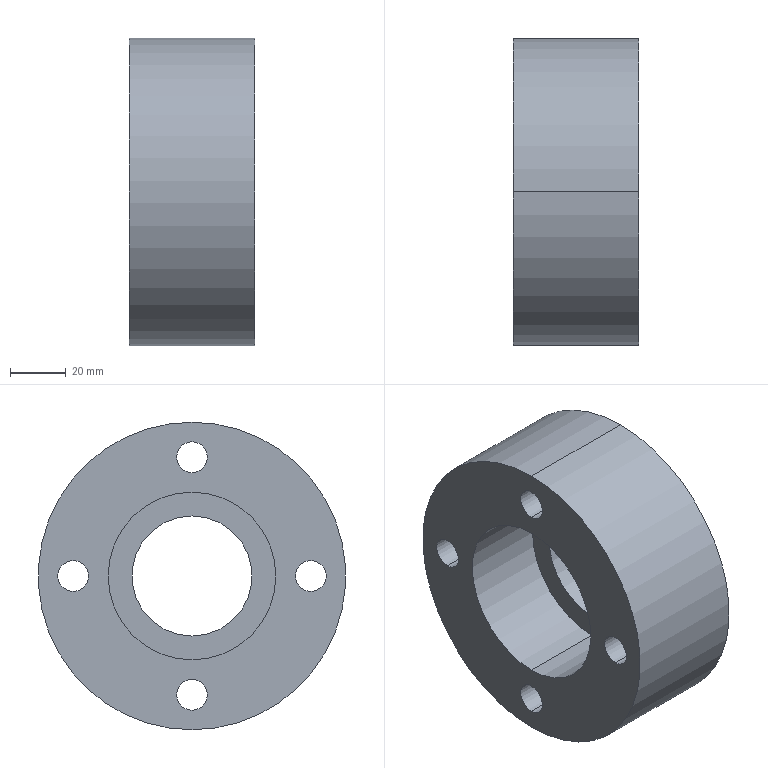Part | SolidWorks | features HoleWzd 1, Revolution 1 | 1 solid | 29 faces | box 45 x 110 x 110 mm | volume 290495 mm3 | cylinder 22 | plane 7 | commonest cylinder face diameters 11 x8 18 x8 43 x2 60 x2 110 x2
STEP:
#1=CARTESIAN_POINT('',(43.415,42.5,9.));
#2=VERTEX_POINT('',#1);
#3=CARTESIAN_POINT('',(43.415,42.5,-9.));
#4=VERTEX_POINT('',#3);
#5=CARTESIAN_POINT('',(43.415,42.5,0.));
#6=DIRECTION('',(1.,0.,0.));
#7=DIRECTION('',(0.,0.,-1.));
#8=AXIS2_PLACEMENT_3D('',#5,#6,#7);
#9=CIRCLE('',#8,9.);
#10=EDGE_CURVE('',#2,#4,#9,.T.);
#11=ORIENTED_EDGE('',*,*,#10,.F.);
#12=CARTESIAN_POINT('',(63.415,42.5,9.));
#13=VERTEX_POINT('',#12);
#14=CARTESIAN_POINT('',(63.415,42.5,9.));
#15=DIRECTION('',(1.,0.,0.));
#16=VECTOR('',#15,1000.);
#17=LINE('',#14,#16);
#18=EDGE_CURVE('',#2,#13,#17,.T.);
#19=ORIENTED_EDGE('',*,*,#18,.T.);
#20=CARTESIAN_POINT('',(63.415,42.5,-9.));
#21=VERTEX_POINT('',#20);
#22=CARTESIAN_POINT('',(63.415,42.5,0.));
#23=DIRECTION('',(1.,0.,0.));
#24=DIRECTION('',(0.,0.,-1.));
#25=AXIS2_PLACEMENT_3D('',#22,#23,#24);
#26=CIRCLE('',#25,9.);
#27=EDGE_CURVE('',#13,#21,#26,.T.);
#28=ORIENTED_EDGE('',*,*,#27,.T.);
#29=CARTESIAN_POINT('',(63.415,42.5,-9.));
#30=DIRECTION('',(1.,0.,0.));
#31=VECTOR('',#30,1000.);
#32=LINE('',#29,#31);
#33=EDGE_CURVE('',#4,#21,#32,.T.);
#34=ORIENTED_EDGE('',*,*,#33,.F.);
#35=EDGE_LOOP('',(#11,#19,#28,#34));
#36=FACE_OUTER_BOUND('',#35,.T.);
#37=CARTESIAN_POINT('',(63.415,42.5,0.));
#38=DIRECTION('',(1.,0.,0.));
#39=DIRECTION('',(0.,0.,-1.));
#40=AXIS2_PLACEMENT_3D('',#37,#38,#39);
#41=CYLINDRICAL_SURFACE('',#40,9.);
#42=ADVANCED_FACE('',(#36),#41,.F.);
#43=CARTESIAN_POINT('',(18.415,42.5,5.5));
#44=VERTEX_POINT('',#43);
#45=CARTESIAN_POINT('',(18.415,42.5,-5.5));
#46=VERTEX_POINT('',#45);
#47=CARTESIAN_POINT('',(18.415,42.5,0.));
#48=DIRECTION('',(1.,0.,0.));
#49=DIRECTION('',(0.,0.,-1.));
#50=AXIS2_PLACEMENT_3D('',#47,#48,#49);
#51=CIRCLE('',#50,5.5);
#52=EDGE_CURVE('',#44,#46,#51,.T.);
#53=ORIENTED_EDGE('',*,*,#52,.F.);
#54=CARTESIAN_POINT('',(43.415,42.5,5.5));
#55=VERTEX_POINT('',#54);
#56=CARTESIAN_POINT('',(63.415,42.5,5.5));
#57=DIRECTION('',(1.,0.,0.));
#58=VECTOR('',#57,1000.);
#59=LINE('',#56,#58);
#60=EDGE_CURVE('',#44,#55,#59,.T.);
#61=ORIENTED_EDGE('',*,*,#60,.T.);
#62=CARTESIAN_POINT('',(43.415,42.5,-5.5));
#63=VERTEX_POINT('',#62);
#64=CARTESIAN_POINT('',(43.415,42.5,0.));
#65=DIRECTION('',(1.,0.,0.));
#66=DIRECTION('',(0.,0.,-1.));
#67=AXIS2_PLACEMENT_3D('',#64,#65,#66);
#68=CIRCLE('',#67,5.5);
#69=EDGE_CURVE('',#55,#63,#68,.T.);
#70=ORIENTED_EDGE('',*,*,#69,.T.);
#71=CARTESIAN_POINT('',(63.415,42.5,-5.5));
#72=DIRECTION('',(1.,0.,0.));
#73=VECTOR('',#72,1000.);
#74=LINE('',#71,#73);
#75=EDGE_CURVE('',#46,#63,#74,.T.);
#76=ORIENTED_EDGE('',*,*,#75,.F.);
#77=EDGE_LOOP('',(#53,#61,#70,#76));
#78=FACE_OUTER_BOUND('',#77,.T.);
#79=CARTESIAN_POINT('',(63.415,42.5,0.));
#80=DIRECTION('',(1.,0.,0.));
#81=DIRECTION('',(0.,0.,-1.));
#82=AXIS2_PLACEMENT_3D('',#79,#80,#81);
#83=CYLINDRICAL_SURFACE('',#82,5.5);
#84=ADVANCED_FACE('',(#78),#83,.F.);
#85=CARTESIAN_POINT('',(43.415,-42.5,9.));
#86=VERTEX_POINT('',#85);
#87=CARTESIAN_POINT('',(43.415,-42.5,-9.));
#88=VERTEX_POINT('',#87);
#89=CARTESIAN_POINT('',(43.415,-42.5,0.));
#90=DIRECTION('',(1.,0.,0.));
#91=DIRECTION('',(0.,0.,-1.));
#92=AXIS2_PLACEMENT_3D('',#89,#90,#91);
#93=CIRCLE('',#92,9.);
#94=EDGE_CURVE('',#86,#88,#93,.T.);
#95=ORIENTED_EDGE('',*,*,#94,.F.);
#96=CARTESIAN_POINT('',(63.415,-42.5,9.));
#97=VERTEX_POINT('',#96);
#98=CARTESIAN_POINT('',(63.415,-42.5,9.));
#99=DIRECTION('',(1.,0.,0.));
#100=VECTOR('',#99,1000.);
#101=LINE('',#98,#100);
#102=EDGE_CURVE('',#86,#97,#101,.T.);
#103=ORIENTED_EDGE('',*,*,#102,.T.);
#104=CARTESIAN_POINT('',(63.415,-42.5,-9.));
#105=VERTEX_POINT('',#104);
#106=CARTESIAN_POINT('',(63.415,-42.5,0.));
#107=DIRECTION('',(1.,0.,0.));
#108=DIRECTION('',(0.,0.,-1.));
#109=AXIS2_PLACEMENT_3D('',#106,#107,#108);
#110=CIRCLE('',#109,9.);
#111=EDGE_CURVE('',#97,#105,#110,.T.);
#112=ORIENTED_EDGE('',*,*,#111,.T.);
#113=CARTESIAN_POINT('',(63.415,-42.5,-9.));
#114=DIRECTION('',(1.,0.,0.));
#115=VECTOR('',#114,1000.);
#116=LINE('',#113,#115);
#117=EDGE_CURVE('',#88,#105,#116,.T.);
#118=ORIENTED_EDGE('',*,*,#117,.F.);
#119=EDGE_LOOP('',(#95,#103,#112,#118));
#120=FACE_OUTER_BOUND('',#119,.T.);
#121=CARTESIAN_POINT('',(63.415,-42.5,0.));
#122=DIRECTION('',(1.,0.,0.));
#123=DIRECTION('',(0.,0.,-1.));
#124=AXIS2_PLACEMENT_3D('',#121,#122,#123);
#125=CYLINDRICAL_SURFACE('',#124,9.);
#126=ADVANCED_FACE('',(#120),#125,.F.);
#127=CARTESIAN_POINT('',(18.415,-42.5,5.5));
#128=VERTEX_POINT('',#127);
#129=CARTESIAN_POINT('',(18.415,-42.5,-5.5));
#130=VERTEX_POINT('',#129);
#131=CARTESIAN_POINT('',(18.415,-42.5,0.));
#132=DIRECTION('',(1.,0.,0.));
#133=DIRECTION('',(0.,0.,-1.));
#134=AXIS2_PLACEMENT_3D('',#131,#132,#133);
#135=CIRCLE('',#134,5.5);
#136=EDGE_CURVE('',#128,#130,#135,.T.);
#137=ORIENTED_EDGE('',*,*,#136,.F.);
#138=CARTESIAN_POINT('',(43.415,-42.5,5.5));
#139=VERTEX_POINT('',#138);
#140=CARTESIAN_POINT('',(63.415,-42.5,5.5));
#141=DIRECTION('',(1.,0.,0.));
#142=VECTOR('',#141,1000.);
#143=LINE('',#140,#142);
#144=EDGE_CURVE('',#128,#139,#143,.T.);
#145=ORIENTED_EDGE('',*,*,#144,.T.);
#146=CARTESIAN_POINT('',(43.415,-42.5,-5.5));
#147=VERTEX_POINT('',#146);
#148=CARTESIAN_POINT('',(43.415,-42.5,0.));
#149=DIRECTION('',(1.,0.,0.));
#150=DIRECTION('',(0.,0.,-1.));
#151=AXIS2_PLACEMENT_3D('',#148,#149,#150);
#152=CIRCLE('',#151,5.5);
#153=EDGE_CURVE('',#139,#147,#152,.T.);
#154=ORIENTED_EDGE('',*,*,#153,.T.);
#155=CARTESIAN_POINT('',(63.415,-42.5,-5.5));
#156=DIRECTION('',(1.,0.,0.));
#157=VECTOR('',#156,1000.);
#158=LINE('',#155,#157);
#159=EDGE_CURVE('',#130,#147,#158,.T.);
#160=ORIENTED_EDGE('',*,*,#159,.F.);
#161=EDGE_LOOP('',(#137,#145,#154,#160));
#162=FACE_OUTER_BOUND('',#161,.T.);
#163=CARTESIAN_POINT('',(63.415,-42.5,0.));
#164=DIRECTION('',(1.,0.,0.));
#165=DIRECTION('',(0.,0.,-1.));
#166=AXIS2_PLACEMENT_3D('',#163,#164,#165);
#167=CYLINDRICAL_SURFACE('',#166,5.5);
#168=ADVANCED_FACE('',(#162),#167,.F.);
#169=CARTESIAN_POINT('',(43.415,0.,51.5));
#170=VERTEX_POINT('',#169);
#171=CARTESIAN_POINT('',(43.415,0.,33.5));
#172=VERTEX_POINT('',#171);
#173=CARTESIAN_POINT('',(43.415,0.,42.5));
#174=DIRECTION('',(1.,0.,0.));
#175=DIRECTION('',(0.,0.,-1.));
#176=AXIS2_PLACEMENT_3D('',#173,#174,#175);
#177=CIRCLE('',#176,9.);
#178=EDGE_CURVE('',#170,#172,#177,.T.);
#179=ORIENTED_EDGE('',*,*,#178,.F.);
#180=CARTESIAN_POINT('',(63.415,0.,51.5));
#181=VERTEX_POINT('',#180);
#182=CARTESIAN_POINT('',(63.415,0.,51.5));
#183=DIRECTION('',(1.,0.,0.));
#184=VECTOR('',#183,1000.);
#185=LINE('',#182,#184);
#186=EDGE_CURVE('',#170,#181,#185,.T.);
#187=ORIENTED_EDGE('',*,*,#186,.T.);
#188=CARTESIAN_POINT('',(63.415,0.,33.5));
#189=VERTEX_POINT('',#188);
#190=CARTESIAN_POINT('',(63.415,0.,42.5));
#191=DIRECTION('',(1.,0.,0.));
#192=DIRECTION('',(0.,0.,-1.));
#193=AXIS2_PLACEMENT_3D('',#190,#191,#192);
#194=CIRCLE('',#193,9.);
#195=EDGE_CURVE('',#181,#189,#194,.T.);
#196=ORIENTED_EDGE('',*,*,#195,.T.);
#197=CARTESIAN_POINT('',(63.415,0.,33.5));
#198=DIRECTION('',(1.,0.,0.));
#199=VECTOR('',#198,1000.);
#200=LINE('',#197,#199);
#201=EDGE_CURVE('',#172,#189,#200,.T.);
#202=ORIENTED_EDGE('',*,*,#201,.F.);
#203=EDGE_LOOP('',(#179,#187,#196,#202));
#204=FACE_OUTER_BOUND('',#203,.T.);
#205=CARTESIAN_POINT('',(63.415,0.,42.5));
#206=DIRECTION('',(1.,0.,0.));
#207=DIRECTION('',(0.,0.,-1.));
#208=AXIS2_PLACEMENT_3D('',#205,#206,#207);
#209=CYLINDRICAL_SURFACE('',#208,9.);
#210=ADVANCED_FACE('',(#204),#209,.F.);
#211=CARTESIAN_POINT('',(18.415,0.,48.));
#212=VERTEX_POINT('',#211);
#213=CARTESIAN_POINT('',(18.415,0.,37.));
#214=VERTEX_POINT('',#213);
#215=CARTESIAN_POINT('',(18.415,0.,42.5));
#216=DIRECTION('',(1.,0.,0.));
#217=DIRECTION('',(0.,0.,-1.));
#218=AXIS2_PLACEMENT_3D('',#215,#216,#217);
#219=CIRCLE('',#218,5.5);
#220=EDGE_CURVE('',#212,#214,#219,.T.);
#221=ORIENTED_EDGE('',*,*,#220,.F.);
#222=CARTESIAN_POINT('',(43.415,0.,48.));
#223=VERTEX_POINT('',#222);
#224=CARTESIAN_POINT('',(63.415,0.,48.));
#225=DIRECTION('',(1.,0.,0.));
#226=VECTOR('',#225,1000.);
#227=LINE('',#224,#226);
#228=EDGE_CURVE('',#212,#223,#227,.T.);
#229=ORIENTED_EDGE('',*,*,#228,.T.);
#230=CARTESIAN_POINT('',(43.415,0.,37.));
#231=VERTEX_POINT('',#230);
#232=CARTESIAN_POINT('',(43.415,0.,42.5));
#233=DIRECTION('',(1.,0.,0.));
#234=DIRECTION('',(0.,0.,-1.));
#235=AXIS2_PLACEMENT_3D('',#232,#233,#234);
#236=CIRCLE('',#235,5.5);
#237=EDGE_CURVE('',#223,#231,#236,.T.);
#238=ORIENTED_EDGE('',*,*,#237,.T.);
#239=CARTESIAN_POINT('',(63.415,0.,37.));
#240=DIRECTION('',(1.,0.,0.));
#241=VECTOR('',#240,1000.);
#242=LINE('',#239,#241);
#243=EDGE_CURVE('',#214,#231,#242,.T.);
#244=ORIENTED_EDGE('',*,*,#243,.F.);
#245=EDGE_LOOP('',(#221,#229,#238,#244));
#246=FACE_OUTER_BOUND('',#245,.T.);
#247=CARTESIAN_POINT('',(63.415,0.,42.5));
#248=DIRECTION('',(1.,0.,0.));
#249=DIRECTION('',(0.,0.,-1.));
#250=AXIS2_PLACEMENT_3D('',#247,#248,#249);
#251=CYLINDRICAL_SURFACE('',#250,5.5);
#252=ADVANCED_FACE('',(#246),#251,.F.);
#253=CARTESIAN_POINT('',(43.415,0.,-33.5));
#254=VERTEX_POINT('',#253);
#255=CARTESIAN_POINT('',(43.415,0.,-51.5));
#256=VERTEX_POINT('',#255);
#257=CARTESIAN_POINT('',(43.415,0.,-42.5));
#258=DIRECTION('',(1.,0.,0.));
#259=DIRECTION('',(0.,0.,-1.));
#260=AXIS2_PLACEMENT_3D('',#257,#258,#259);
#261=CIRCLE('',#260,9.);
#262=EDGE_CURVE('',#254,#256,#261,.T.);
#263=ORIENTED_EDGE('',*,*,#262,.F.);
#264=CARTESIAN_POINT('',(63.415,0.,-33.5));
#265=VERTEX_POINT('',#264);
#266=CARTESIAN_POINT('',(63.415,0.,-33.5));
#267=DIRECTION('',(1.,0.,0.));
#268=VECTOR('',#267,1000.);
#269=LINE('',#266,#268);
#270=EDGE_CURVE('',#254,#265,#269,.T.);
#271=ORIENTED_EDGE('',*,*,#270,.T.);
#272=CARTESIAN_POINT('',(63.415,0.,-51.5));
#273=VERTEX_POINT('',#272);
#274=CARTESIAN_POINT('',(63.415,0.,-42.5));
#275=DIRECTION('',(1.,0.,0.));
#276=DIRECTION('',(0.,0.,-1.));
#277=AXIS2_PLACEMENT_3D('',#274,#275,#276);
#278=CIRCLE('',#277,9.);
#279=EDGE_CURVE('',#265,#273,#278,.T.);
#280=ORIENTED_EDGE('',*,*,#279,.T.);
#281=CARTESIAN_POINT('',(63.415,0.,-51.5));
#282=DIRECTION('',(1.,0.,0.));
#283=VECTOR('',#282,1000.);
#284=LINE('',#281,#283);
#285=EDGE_CURVE('',#256,#273,#284,.T.);
#286=ORIENTED_EDGE('',*,*,#285,.F.);
#287=EDGE_LOOP('',(#263,#271,#280,#286));
#288=FACE_OUTER_BOUND('',#287,.T.);
#289=CARTESIAN_POINT('',(63.415,0.,-42.5));
#290=DIRECTION('',(1.,0.,0.));
#291=DIRECTION('',(0.,0.,-1.));
#292=AXIS2_PLACEMENT_3D('',#289,#290,#291);
#293=CYLINDRICAL_SURFACE('',#292,9.);
#294=ADVANCED_FACE('',(#288),#293,.F.);
#295=CARTESIAN_POINT('',(18.415,0.,-37.));
#296=VERTEX_POINT('',#295);
#297=CARTESIAN_POINT('',(18.415,0.,-48.));
#298=VERTEX_POINT('',#297);
#299=CARTESIAN_POINT('',(18.415,0.,-42.5));
#300=DIRECTION('',(1.,0.,0.));
#301=DIRECTION('',(0.,0.,-1.));
#302=AXIS2_PLACEMENT_3D('',#299,#300,#301);
#303=CIRCLE('',#302,5.5);
#304=EDGE_CURVE('',#296,#298,#303,.T.);
#305=ORIENTED_EDGE('',*,*,#304,.F.);
#306=CARTESIAN_POINT('',(43.415,0.,-37.));
#307=VERTEX_POINT('',#306);
#308=CARTESIAN_POINT('',(63.415,0.,-37.));
#309=DIRECTION('',(1.,0.,0.));
#310=VECTOR('',#309,1000.);
#311=LINE('',#308,#310);
#312=EDGE_CURVE('',#296,#307,#311,.T.);
#313=ORIENTED_EDGE('',*,*,#312,.T.);
#314=CARTESIAN_POINT('',(43.415,0.,-48.));
#315=VERTEX_POINT('',#314);
#316=CARTESIAN_POINT('',(43.415,0.,-42.5));
#317=DIRECTION('',(1.,0.,0.));
#318=DIRECTION('',(0.,0.,-1.));
#319=AXIS2_PLACEMENT_3D('',#316,#317,#318);
#320=CIRCLE('',#319,5.5);
#321=EDGE_CURVE('',#307,#315,#320,.T.);
#322=ORIENTED_EDGE('',*,*,#321,.T.);
#323=CARTESIAN_POINT('',(63.415,0.,-48.));
#324=DIRECTION('',(1.,0.,0.));
#325=VECTOR('',#324,1000.);
#326=LINE('',#323,#325);
#327=EDGE_CURVE('',#298,#315,#326,.T.);
#328=ORIENTED_EDGE('',*,*,#327,.F.);
#329=EDGE_LOOP('',(#305,#313,#322,#328));
#330=FACE_OUTER_BOUND('',#329,.T.);
#331=CARTESIAN_POINT('',(63.415,0.,-42.5));
#332=DIRECTION('',(1.,0.,0.));
#333=DIRECTION('',(0.,0.,-1.));
#334=AXIS2_PLACEMENT_3D('',#331,#332,#333);
#335=CYLINDRICAL_SURFACE('',#334,5.5);
#336=ADVANCED_FACE('',(#330),#335,.F.);
#337=CARTESIAN_POINT('',(63.415,0.,55.));
#338=VERTEX_POINT('',#337);
#339=CARTESIAN_POINT('',(63.415,0.,-55.));
#340=VERTEX_POINT('',#339);
#341=CARTESIAN_POINT('',(63.415,0.,0.));
#342=DIRECTION('',(-1.,0.,0.));
#343=DIRECTION('',(0.,0.,1.));
#344=AXIS2_PLACEMENT_3D('',#341,#342,#343);
#345=CIRCLE('',#344,55.);
#346=EDGE_CURVE('',#338,#340,#345,.T.);
#347=ORIENTED_EDGE('',*,*,#346,.T.);
#348=CARTESIAN_POINT('',(18.415,0.,-55.));
#349=VERTEX_POINT('',#348);
#350=CARTESIAN_POINT('',(0.,0.,-55.));
#351=DIRECTION('',(-1.,0.,0.));
#352=VECTOR('',#351,1000.);
#353=LINE('',#350,#352);
#354=EDGE_CURVE('',#340,#349,#353,.T.);
#355=ORIENTED_EDGE('',*,*,#354,.T.);
#356=CARTESIAN_POINT('',(18.415,0.,55.));
#357=VERTEX_POINT('',#356);
#358=CARTESIAN_POINT('',(18.415,0.,0.));
#359=DIRECTION('',(-1.,0.,0.));
#360=DIRECTION('',(0.,0.,1.));
#361=AXIS2_PLACEMENT_3D('',#358,#359,#360);
#362=CIRCLE('',#361,55.);
#363=EDGE_CURVE('',#357,#349,#362,.T.);
#364=ORIENTED_EDGE('',*,*,#363,.F.);
#365=CARTESIAN_POINT('',(0.,0.,55.));
#366=DIRECTION('',(-1.,0.,0.));
#367=VECTOR('',#366,1000.);
#368=LINE('',#365,#367);
#369=EDGE_CURVE('',#338,#357,#368,.T.);
#370=ORIENTED_EDGE('',*,*,#369,.F.);
#371=EDGE_LOOP('',(#347,#355,#364,#370));
#372=FACE_OUTER_BOUND('',#371,.T.);
#373=CARTESIAN_POINT('',(0.,0.,0.));
#374=DIRECTION('',(-1.,0.,0.));
#375=DIRECTION('',(0.,0.,1.));
#376=AXIS2_PLACEMENT_3D('',#373,#374,#375);
#377=CYLINDRICAL_SURFACE('',#376,55.);
#378=ADVANCED_FACE('',(#372),#377,.T.);
#379=CARTESIAN_POINT('',(48.915,0.,-30.));
#380=VERTEX_POINT('',#379);
#381=CARTESIAN_POINT('',(48.915,0.,30.));
#382=VERTEX_POINT('',#381);
#383=CARTESIAN_POINT('',(48.915,0.,0.));
#384=DIRECTION('',(-1.,0.,0.));
#385=DIRECTION('',(0.,0.,1.));
#386=AXIS2_PLACEMENT_3D('',#383,#384,#385);
#387=CIRCLE('',#386,30.);
#388=EDGE_CURVE('',#380,#382,#387,.T.);
#389=ORIENTED_EDGE('',*,*,#388,.F.);
#390=CARTESIAN_POINT('',(18.415,0.,-30.));
#391=VERTEX_POINT('',#390);
#392=CARTESIAN_POINT('',(0.,0.,-30.));
#393=DIRECTION('',(-1.,0.,0.));
#394=VECTOR('',#393,1000.);
#395=LINE('',#392,#394);
#396=EDGE_CURVE('',#380,#391,#395,.T.);
#397=ORIENTED_EDGE('',*,*,#396,.T.);
#398=CARTESIAN_POINT('',(18.415,0.,30.));
#399=VERTEX_POINT('',#398);
#400=CARTESIAN_POINT('',(18.415,0.,0.));
#401=DIRECTION('',(-1.,0.,0.));
#402=DIRECTION('',(0.,0.,1.));
#403=AXIS2_PLACEMENT_3D('',#400,#401,#402);
#404=CIRCLE('',#403,30.);
#405=EDGE_CURVE('',#391,#399,#404,.T.);
#406=ORIENTED_EDGE('',*,*,#405,.T.);
#407=CARTESIAN_POINT('',(0.,0.,30.));
#408=DIRECTION('',(-1.,0.,0.));
#409=VECTOR('',#408,1000.);
#410=LINE('',#407,#409);
#411=EDGE_CURVE('',#382,#399,#410,.T.);
#412=ORIENTED_EDGE('',*,*,#411,.F.);
#413=EDGE_LOOP('',(#389,#397,#406,#412));
#414=FACE_OUTER_BOUND('',#413,.T.);
#415=CARTESIAN_POINT('',(0.,0.,0.));
#416=DIRECTION('',(-1.,0.,0.));
#417=DIRECTION('',(0.,0.,1.));
#418=AXIS2_PLACEMENT_3D('',#415,#416,#417);
#419=CYLINDRICAL_SURFACE('',#418,30.);
#420=ADVANCED_FACE('',(#414),#419,.F.);
#421=CARTESIAN_POINT('',(63.415,0.,-21.5));
#422=VERTEX_POINT('',#421);
#423=CARTESIAN_POINT('',(63.415,0.,21.5));
#424=VERTEX_POINT('',#423);
#425=CARTESIAN_POINT('',(63.415,0.,0.));
#426=DIRECTION('',(-1.,0.,0.));
#427=DIRECTION('',(0.,0.,1.));
#428=AXIS2_PLACEMENT_3D('',#425,#426,#427);
#429=CIRCLE('',#428,21.5);
#430=EDGE_CURVE('',#422,#424,#429,.T.);
#431=ORIENTED_EDGE('',*,*,#430,.F.);
#432=CARTESIAN_POINT('',(48.915,0.,-21.5));
#433=VERTEX_POINT('',#432);
#434=CARTESIAN_POINT('',(0.,0.,-21.5));
#435=DIRECTION('',(-1.,0.,0.));
#436=VECTOR('',#435,1000.);
#437=LINE('',#434,#436);
#438=EDGE_CURVE('',#422,#433,#437,.T.);
#439=ORIENTED_EDGE('',*,*,#438,.T.);
#440=CARTESIAN_POINT('',(48.915,0.,21.5));
#441=VERTEX_POINT('',#440);
#442=CARTESIAN_POINT('',(48.915,0.,0.));
#443=DIRECTION('',(-1.,0.,0.));
#444=DIRECTION('',(0.,0.,1.));
#445=AXIS2_PLACEMENT_3D('',#442,#443,#444);
#446=CIRCLE('',#445,21.5);
#447=EDGE_CURVE('',#433,#441,#446,.T.);
#448=ORIENTED_EDGE('',*,*,#447,.T.);
#449=CARTESIAN_POINT('',(0.,0.,21.5));
#450=DIRECTION('',(-1.,0.,0.));
#451=VECTOR('',#450,1000.);
#452=LINE('',#449,#451);
#453=EDGE_CURVE('',#424,#441,#452,.T.);
#454=ORIENTED_EDGE('',*,*,#453,.F.);
#455=EDGE_LOOP('',(#431,#439,#448,#454));
#456=FACE_OUTER_BOUND('',#455,.T.);
#457=CARTESIAN_POINT('',(0.,0.,0.));
#458=DIRECTION('',(-1.,0.,0.));
#459=DIRECTION('',(0.,0.,1.));
#460=AXIS2_PLACEMENT_3D('',#457,#458,#459);
#461=CYLINDRICAL_SURFACE('',#460,21.5);
#462=ADVANCED_FACE('',(#456),#461,.F.);
#463=CARTESIAN_POINT('',(63.415,42.5,0.));
#464=DIRECTION('',(1.,0.,0.));
#465=DIRECTION('',(0.,0.,-1.));
#466=AXIS2_PLACEMENT_3D('',#463,#464,#465);
#467=CIRCLE('',#466,9.);
#468=EDGE_CURVE('',#21,#13,#467,.T.);
#469=ORIENTED_EDGE('',*,*,#468,.F.);
#470=ORIENTED_EDGE('',*,*,#27,.F.);
#471=EDGE_LOOP('',(#469,#470));
#472=FACE_BOUND('',#471,.T.);
#473=CARTESIAN_POINT('',(63.415,-42.5,0.));
#474=DIRECTION('',(1.,0.,0.));
#475=DIRECTION('',(0.,0.,-1.));
#476=AXIS2_PLACEMENT_3D('',#473,#474,#475);
#477=CIRCLE('',#476,9.);
#478=EDGE_CURVE('',#105,#97,#477,.T.);
#479=ORIENTED_EDGE('',*,*,#478,.F.);
#480=ORIENTED_EDGE('',*,*,#111,.F.);
#481=EDGE_LOOP('',(#479,#480));
#482=FACE_BOUND('',#481,.T.);
#483=CARTESIAN_POINT('',(63.415,0.,42.5));
#484=DIRECTION('',(1.,0.,0.));
#485=DIRECTION('',(0.,0.,-1.));
#486=AXIS2_PLACEMENT_3D('',#483,#484,#485);
#487=CIRCLE('',#486,9.);
#488=EDGE_CURVE('',#189,#181,#487,.T.);
#489=ORIENTED_EDGE('',*,*,#488,.F.);
#490=ORIENTED_EDGE('',*,*,#195,.F.);
#491=EDGE_LOOP('',(#489,#490));
#492=FACE_BOUND('',#491,.T.);
#493=CARTESIAN_POINT('',(63.415,0.,-42.5));
#494=DIRECTION('',(1.,0.,0.));
#495=DIRECTION('',(0.,0.,-1.));
#496=AXIS2_PLACEMENT_3D('',#493,#494,#495);
#497=CIRCLE('',#496,9.);
#498=EDGE_CURVE('',#273,#265,#497,.T.);
#499=ORIENTED_EDGE('',*,*,#498,.F.);
#500=ORIENTED_EDGE('',*,*,#279,.F.);
#501=EDGE_LOOP('',(#499,#500));
#502=FACE_BOUND('',#501,.T.);
#503=ORIENTED_EDGE('',*,*,#346,.F.);
#504=CARTESIAN_POINT('',(63.415,0.,0.));
#505=DIRECTION('',(-1.,0.,0.));
#506=DIRECTION('',(0.,0.,1.));
#507=AXIS2_PLACEMENT_3D('',#504,#505,#506);
#508=CIRCLE('',#507,55.);
#509=EDGE_CURVE('',#340,#338,#508,.T.);
#510=ORIENTED_EDGE('',*,*,#509,.F.);
#511=EDGE_LOOP('',(#503,#510));
#512=FACE_OUTER_BOUND('',#511,.T.);
#513=CARTESIAN_POINT('',(63.415,0.,0.));
#514=DIRECTION('',(-1.,0.,0.));
#515=DIRECTION('',(0.,0.,1.));
#516=AXIS2_PLACEMENT_3D('',#513,#514,#515);
#517=CIRCLE('',#516,21.5);
#518=EDGE_CURVE('',#424,#422,#517,.T.);
#519=ORIENTED_EDGE('',*,*,#518,.T.);
#520=ORIENTED_EDGE('',*,*,#430,.T.);
#521=EDGE_LOOP('',(#519,#520));
#522=FACE_BOUND('',#521,.T.);
#523=CARTESIAN_POINT('',(63.415,21.5,0.));
#524=DIRECTION('',(-1.,0.,0.));
#525=DIRECTION('',(0.,0.,1.));
#526=AXIS2_PLACEMENT_3D('',#523,#524,#525);
#527=PLANE('',#526);
#528=ADVANCED_FACE('',(#472,#482,#492,#502,#512,#522),#527,.F.);
#529=ORIENTED_EDGE('',*,*,#438,.F.);
#530=ORIENTED_EDGE('',*,*,#518,.F.);
#531=ORIENTED_EDGE('',*,*,#453,.T.);
#532=CARTESIAN_POINT('',(48.915,0.,0.));
#533=DIRECTION('',(-1.,0.,0.));
#534=DIRECTION('',(0.,0.,1.));
#535=AXIS2_PLACEMENT_3D('',#532,#533,#534);
#536=CIRCLE('',#535,21.5);
#537=EDGE_CURVE('',#441,#433,#536,.T.);
#538=ORIENTED_EDGE('',*,*,#537,.T.);
#539=EDGE_LOOP('',(#529,#530,#531,#538));
#540=FACE_OUTER_BOUND('',#539,.T.);
#541=CARTESIAN_POINT('',(0.,0.,0.));
#542=DIRECTION('',(-1.,0.,0.));
#543=DIRECTION('',(0.,0.,1.));
#544=AXIS2_PLACEMENT_3D('',#541,#542,#543);
#545=CYLINDRICAL_SURFACE('',#544,21.5);
#546=ADVANCED_FACE('',(#540),#545,.F.);
#547=ORIENTED_EDGE('',*,*,#537,.F.);
#548=ORIENTED_EDGE('',*,*,#447,.F.);
#549=EDGE_LOOP('',(#547,#548));
#550=FACE_BOUND('',#549,.T.);
#551=CARTESIAN_POINT('',(48.915,0.,0.));
#552=DIRECTION('',(-1.,0.,0.));
#553=DIRECTION('',(0.,0.,1.));
#554=AXIS2_PLACEMENT_3D('',#551,#552,#553);
#555=CIRCLE('',#554,30.);
#556=EDGE_CURVE('',#382,#380,#555,.T.);
#557=ORIENTED_EDGE('',*,*,#556,.T.);
#558=ORIENTED_EDGE('',*,*,#388,.T.);
#559=EDGE_LOOP('',(#557,#558));
#560=FACE_OUTER_BOUND('',#559,.T.);
#561=CARTESIAN_POINT('',(48.915,21.5,0.));
#562=DIRECTION('',(1.,0.,0.));
#563=DIRECTION('',(0.,0.,-1.));
#564=AXIS2_PLACEMENT_3D('',#561,#562,#563);
#565=PLANE('',#564);
#566=ADVANCED_FACE('',(#550,#560),#565,.F.);
#567=ORIENTED_EDGE('',*,*,#396,.F.);
#568=ORIENTED_EDGE('',*,*,#556,.F.);
#569=ORIENTED_EDGE('',*,*,#411,.T.);
#570=CARTESIAN_POINT('',(18.415,0.,0.));
#571=DIRECTION('',(-1.,0.,0.));
#572=DIRECTION('',(0.,0.,1.));
#573=AXIS2_PLACEMENT_3D('',#570,#571,#572);
#574=CIRCLE('',#573,30.);
#575=EDGE_CURVE('',#399,#391,#574,.T.);
#576=ORIENTED_EDGE('',*,*,#575,.T.);
#577=EDGE_LOOP('',(#567,#568,#569,#576));
#578=FACE_OUTER_BOUND('',#577,.T.);
#579=CARTESIAN_POINT('',(0.,0.,0.));
#580=DIRECTION('',(-1.,0.,0.));
#581=DIRECTION('',(0.,0.,1.));
#582=AXIS2_PLACEMENT_3D('',#579,#580,#581);
#583=CYLINDRICAL_SURFACE('',#582,30.);
#584=ADVANCED_FACE('',(#578),#583,.F.);
#585=CARTESIAN_POINT('',(18.415,42.5,0.));
#586=DIRECTION('',(1.,0.,0.));
#587=DIRECTION('',(0.,0.,-1.));
#588=AXIS2_PLACEMENT_3D('',#585,#586,#587);
#589=CIRCLE('',#588,5.5);
#590=EDGE_CURVE('',#46,#44,#589,.T.);
#591=ORIENTED_EDGE('',*,*,#590,.T.);
#592=ORIENTED_EDGE('',*,*,#52,.T.);
#593=EDGE_LOOP('',(#591,#592));
#594=FACE_BOUND('',#593,.T.);
#595=CARTESIAN_POINT('',(18.415,-42.5,0.));
#596=DIRECTION('',(1.,0.,0.));
#597=DIRECTION('',(0.,0.,-1.));
#598=AXIS2_PLACEMENT_3D('',#595,#596,#597);
#599=CIRCLE('',#598,5.5);
#600=EDGE_CURVE('',#130,#128,#599,.T.);
#601=ORIENTED_EDGE('',*,*,#600,.T.);
#602=ORIENTED_EDGE('',*,*,#136,.T.);
#603=EDGE_LOOP('',(#601,#602));
#604=FACE_BOUND('',#603,.T.);
#605=CARTESIAN_POINT('',(18.415,0.,42.5));
#606=DIRECTION('',(1.,0.,0.));
#607=DIRECTION('',(0.,0.,-1.));
#608=AXIS2_PLACEMENT_3D('',#605,#606,#607);
#609=CIRCLE('',#608,5.5);
#610=EDGE_CURVE('',#214,#212,#609,.T.);
#611=ORIENTED_EDGE('',*,*,#610,.T.);
#612=ORIENTED_EDGE('',*,*,#220,.T.);
#613=EDGE_LOOP('',(#611,#612));
#614=FACE_BOUND('',#613,.T.);
#615=CARTESIAN_POINT('',(18.415,0.,-42.5));
#616=DIRECTION('',(1.,0.,0.));
#617=DIRECTION('',(0.,0.,-1.));
#618=AXIS2_PLACEMENT_3D('',#615,#616,#617);
#619=CIRCLE('',#618,5.5);
#620=EDGE_CURVE('',#298,#296,#619,.T.);
#621=ORIENTED_EDGE('',*,*,#620,.T.);
#622=ORIENTED_EDGE('',*,*,#304,.T.);
#623=EDGE_LOOP('',(#621,#622));
#624=FACE_BOUND('',#623,.T.);
#625=ORIENTED_EDGE('',*,*,#575,.F.);
#626=ORIENTED_EDGE('',*,*,#405,.F.);
#627=EDGE_LOOP('',(#625,#626));
#628=FACE_BOUND('',#627,.T.);
#629=ORIENTED_EDGE('',*,*,#363,.T.);
#630=CARTESIAN_POINT('',(18.415,0.,0.));
#631=DIRECTION('',(-1.,0.,0.));
#632=DIRECTION('',(0.,0.,1.));
#633=AXIS2_PLACEMENT_3D('',#630,#631,#632);
#634=CIRCLE('',#633,55.);
#635=EDGE_CURVE('',#349,#357,#634,.T.);
#636=ORIENTED_EDGE('',*,*,#635,.T.);
#637=EDGE_LOOP('',(#629,#636));
#638=FACE_OUTER_BOUND('',#637,.T.);
#639=CARTESIAN_POINT('',(18.415,30.,0.));
#640=DIRECTION('',(1.,0.,0.));
#641=DIRECTION('',(0.,0.,-1.));
#642=AXIS2_PLACEMENT_3D('',#639,#640,#641);
#643=PLANE('',#642);
#644=ADVANCED_FACE('',(#594,#604,#614,#624,#628,#638),#643,.F.);
#645=ORIENTED_EDGE('',*,*,#354,.F.);
#646=ORIENTED_EDGE('',*,*,#509,.T.);
#647=ORIENTED_EDGE('',*,*,#369,.T.);
#648=ORIENTED_EDGE('',*,*,#635,.F.);
#649=EDGE_LOOP('',(#645,#646,#647,#648));
#650=FACE_OUTER_BOUND('',#649,.T.);
#651=CARTESIAN_POINT('',(0.,0.,0.));
#652=DIRECTION('',(-1.,0.,0.));
#653=DIRECTION('',(0.,0.,1.));
#654=AXIS2_PLACEMENT_3D('',#651,#652,#653);
#655=CYLINDRICAL_SURFACE('',#654,55.);
#656=ADVANCED_FACE('',(#650),#655,.T.);
#657=ORIENTED_EDGE('',*,*,#312,.F.);
#658=ORIENTED_EDGE('',*,*,#620,.F.);
#659=ORIENTED_EDGE('',*,*,#327,.T.);
#660=CARTESIAN_POINT('',(43.415,0.,-42.5));
#661=DIRECTION('',(1.,0.,0.));
#662=DIRECTION('',(0.,0.,-1.));
#663=AXIS2_PLACEMENT_3D('',#660,#661,#662);
#664=CIRCLE('',#663,5.5);
#665=EDGE_CURVE('',#315,#307,#664,.T.);
#666=ORIENTED_EDGE('',*,*,#665,.T.);
#667=EDGE_LOOP('',(#657,#658,#659,#666));
#668=FACE_OUTER_BOUND('',#667,.T.);
#669=CARTESIAN_POINT('',(63.415,0.,-42.5));
#670=DIRECTION('',(1.,0.,0.));
#671=DIRECTION('',(0.,0.,-1.));
#672=AXIS2_PLACEMENT_3D('',#669,#670,#671);
#673=CYLINDRICAL_SURFACE('',#672,5.5);
#674=ADVANCED_FACE('',(#668),#673,.F.);
#675=ORIENTED_EDGE('',*,*,#665,.F.);
#676=ORIENTED_EDGE('',*,*,#321,.F.);
#677=EDGE_LOOP('',(#675,#676));
#678=FACE_BOUND('',#677,.T.);
#679=CARTESIAN_POINT('',(43.415,0.,-42.5));
#680=DIRECTION('',(1.,0.,0.));
#681=DIRECTION('',(0.,0.,-1.));
#682=AXIS2_PLACEMENT_3D('',#679,#680,#681);
#683=CIRCLE('',#682,9.);
#684=EDGE_CURVE('',#256,#254,#683,.T.);
#685=ORIENTED_EDGE('',*,*,#684,.T.);
#686=ORIENTED_EDGE('',*,*,#262,.T.);
#687=EDGE_LOOP('',(#685,#686));
#688=FACE_OUTER_BOUND('',#687,.T.);
#689=CARTESIAN_POINT('',(43.415,5.5,-42.5));
#690=DIRECTION('',(-1.,0.,0.));
#691=DIRECTION('',(0.,0.,1.));
#692=AXIS2_PLACEMENT_3D('',#689,#690,#691);
#693=PLANE('',#692);
#694=ADVANCED_FACE('',(#678,#688),#693,.F.);
#695=ORIENTED_EDGE('',*,*,#270,.F.);
#696=ORIENTED_EDGE('',*,*,#684,.F.);
#697=ORIENTED_EDGE('',*,*,#285,.T.);
#698=ORIENTED_EDGE('',*,*,#498,.T.);
#699=EDGE_LOOP('',(#695,#696,#697,#698));
#700=FACE_OUTER_BOUND('',#699,.T.);
#701=CARTESIAN_POINT('',(63.415,0.,-42.5));
#702=DIRECTION('',(1.,0.,0.));
#703=DIRECTION('',(0.,0.,-1.));
#704=AXIS2_PLACEMENT_3D('',#701,#702,#703);
#705=CYLINDRICAL_SURFACE('',#704,9.);
#706=ADVANCED_FACE('',(#700),#705,.F.);
#707=ORIENTED_EDGE('',*,*,#228,.F.);
#708=ORIENTED_EDGE('',*,*,#610,.F.);
#709=ORIENTED_EDGE('',*,*,#243,.T.);
#710=CARTESIAN_POINT('',(43.415,0.,42.5));
#711=DIRECTION('',(1.,0.,0.));
#712=DIRECTION('',(0.,0.,-1.));
#713=AXIS2_PLACEMENT_3D('',#710,#711,#712);
#714=CIRCLE('',#713,5.5);
#715=EDGE_CURVE('',#231,#223,#714,.T.);
#716=ORIENTED_EDGE('',*,*,#715,.T.);
#717=EDGE_LOOP('',(#707,#708,#709,#716));
#718=FACE_OUTER_BOUND('',#717,.T.);
#719=CARTESIAN_POINT('',(63.415,0.,42.5));
#720=DIRECTION('',(1.,0.,0.));
#721=DIRECTION('',(0.,0.,-1.));
#722=AXIS2_PLACEMENT_3D('',#719,#720,#721);
#723=CYLINDRICAL_SURFACE('',#722,5.5);
#724=ADVANCED_FACE('',(#718),#723,.F.);
#725=ORIENTED_EDGE('',*,*,#715,.F.);
#726=ORIENTED_EDGE('',*,*,#237,.F.);
#727=EDGE_LOOP('',(#725,#726));
#728=FACE_BOUND('',#727,.T.);
#729=CARTESIAN_POINT('',(43.415,0.,42.5));
#730=DIRECTION('',(1.,0.,0.));
#731=DIRECTION('',(0.,0.,-1.));
#732=AXIS2_PLACEMENT_3D('',#729,#730,#731);
#733=CIRCLE('',#732,9.);
#734=EDGE_CURVE('',#172,#170,#733,.T.);
#735=ORIENTED_EDGE('',*,*,#734,.T.);
#736=ORIENTED_EDGE('',*,*,#178,.T.);
#737=EDGE_LOOP('',(#735,#736));
#738=FACE_OUTER_BOUND('',#737,.T.);
#739=CARTESIAN_POINT('',(43.415,5.5,42.5));
#740=DIRECTION('',(-1.,0.,0.));
#741=DIRECTION('',(0.,0.,1.));
#742=AXIS2_PLACEMENT_3D('',#739,#740,#741);
#743=PLANE('',#742);
#744=ADVANCED_FACE('',(#728,#738),#743,.F.);
#745=ORIENTED_EDGE('',*,*,#186,.F.);
#746=ORIENTED_EDGE('',*,*,#734,.F.);
#747=ORIENTED_EDGE('',*,*,#201,.T.);
#748=ORIENTED_EDGE('',*,*,#488,.T.);
#749=EDGE_LOOP('',(#745,#746,#747,#748));
#750=FACE_OUTER_BOUND('',#749,.T.);
#751=CARTESIAN_POINT('',(63.415,0.,42.5));
#752=DIRECTION('',(1.,0.,0.));
#753=DIRECTION('',(0.,0.,-1.));
#754=AXIS2_PLACEMENT_3D('',#751,#752,#753);
#755=CYLINDRICAL_SURFACE('',#754,9.);
#756=ADVANCED_FACE('',(#750),#755,.F.);
#757=ORIENTED_EDGE('',*,*,#144,.F.);
#758=ORIENTED_EDGE('',*,*,#600,.F.);
#759=ORIENTED_EDGE('',*,*,#159,.T.);
#760=CARTESIAN_POINT('',(43.415,-42.5,0.));
#761=DIRECTION('',(1.,0.,0.));
#762=DIRECTION('',(0.,0.,-1.));
#763=AXIS2_PLACEMENT_3D('',#760,#761,#762);
#764=CIRCLE('',#763,5.5);
#765=EDGE_CURVE('',#147,#139,#764,.T.);
#766=ORIENTED_EDGE('',*,*,#765,.T.);
#767=EDGE_LOOP('',(#757,#758,#759,#766));
#768=FACE_OUTER_BOUND('',#767,.T.);
#769=CARTESIAN_POINT('',(63.415,-42.5,0.));
#770=DIRECTION('',(1.,0.,0.));
#771=DIRECTION('',(0.,0.,-1.));
#772=AXIS2_PLACEMENT_3D('',#769,#770,#771);
#773=CYLINDRICAL_SURFACE('',#772,5.5);
#774=ADVANCED_FACE('',(#768),#773,.F.);
#775=ORIENTED_EDGE('',*,*,#765,.F.);
#776=ORIENTED_EDGE('',*,*,#153,.F.);
#777=EDGE_LOOP('',(#775,#776));
#778=FACE_BOUND('',#777,.T.);
#779=CARTESIAN_POINT('',(43.415,-42.5,0.));
#780=DIRECTION('',(1.,0.,0.));
#781=DIRECTION('',(0.,0.,-1.));
#782=AXIS2_PLACEMENT_3D('',#779,#780,#781);
#783=CIRCLE('',#782,9.);
#784=EDGE_CURVE('',#88,#86,#783,.T.);
#785=ORIENTED_EDGE('',*,*,#784,.T.);
#786=ORIENTED_EDGE('',*,*,#94,.T.);
#787=EDGE_LOOP('',(#785,#786));
#788=FACE_OUTER_BOUND('',#787,.T.);
#789=CARTESIAN_POINT('',(43.415,-37.,0.));
#790=DIRECTION('',(-1.,0.,0.));
#791=DIRECTION('',(0.,0.,1.));
#792=AXIS2_PLACEMENT_3D('',#789,#790,#791);
#793=PLANE('',#792);
#794=ADVANCED_FACE('',(#778,#788),#793,.F.);
#795=ORIENTED_EDGE('',*,*,#102,.F.);
#796=ORIENTED_EDGE('',*,*,#784,.F.);
#797=ORIENTED_EDGE('',*,*,#117,.T.);
#798=ORIENTED_EDGE('',*,*,#478,.T.);
#799=EDGE_LOOP('',(#795,#796,#797,#798));
#800=FACE_OUTER_BOUND('',#799,.T.);
#801=CARTESIAN_POINT('',(63.415,-42.5,0.));
#802=DIRECTION('',(1.,0.,0.));
#803=DIRECTION('',(0.,0.,-1.));
#804=AXIS2_PLACEMENT_3D('',#801,#802,#803);
#805=CYLINDRICAL_SURFACE('',#804,9.);
#806=ADVANCED_FACE('',(#800),#805,.F.);
#807=ORIENTED_EDGE('',*,*,#60,.F.);
#808=ORIENTED_EDGE('',*,*,#590,.F.);
#809=ORIENTED_EDGE('',*,*,#75,.T.);
#810=CARTESIAN_POINT('',(43.415,42.5,0.));
#811=DIRECTION('',(1.,0.,0.));
#812=DIRECTION('',(0.,0.,-1.));
#813=AXIS2_PLACEMENT_3D('',#810,#811,#812);
#814=CIRCLE('',#813,5.5);
#815=EDGE_CURVE('',#63,#55,#814,.T.);
#816=ORIENTED_EDGE('',*,*,#815,.T.);
#817=EDGE_LOOP('',(#807,#808,#809,#816));
#818=FACE_OUTER_BOUND('',#817,.T.);
#819=CARTESIAN_POINT('',(63.415,42.5,0.));
#820=DIRECTION('',(1.,0.,0.));
#821=DIRECTION('',(0.,0.,-1.));
#822=AXIS2_PLACEMENT_3D('',#819,#820,#821);
#823=CYLINDRICAL_SURFACE('',#822,5.5);
#824=ADVANCED_FACE('',(#818),#823,.F.);
#825=ORIENTED_EDGE('',*,*,#815,.F.);
#826=ORIENTED_EDGE('',*,*,#69,.F.);
#827=EDGE_LOOP('',(#825,#826));
#828=FACE_BOUND('',#827,.T.);
#829=CARTESIAN_POINT('',(43.415,42.5,0.));
#830=DIRECTION('',(1.,0.,0.));
#831=DIRECTION('',(0.,0.,-1.));
#832=AXIS2_PLACEMENT_3D('',#829,#830,#831);
#833=CIRCLE('',#832,9.);
#834=EDGE_CURVE('',#4,#2,#833,.T.);
#835=ORIENTED_EDGE('',*,*,#834,.T.);
#836=ORIENTED_EDGE('',*,*,#10,.T.);
#837=EDGE_LOOP('',(#835,#836));
#838=FACE_OUTER_BOUND('',#837,.T.);
#839=CARTESIAN_POINT('',(43.415,48.,0.));
#840=DIRECTION('',(-1.,0.,0.));
#841=DIRECTION('',(0.,0.,1.));
#842=AXIS2_PLACEMENT_3D('',#839,#840,#841);
#843=PLANE('',#842);
#844=ADVANCED_FACE('',(#828,#838),#843,.F.);
#845=ORIENTED_EDGE('',*,*,#18,.F.);
#846=ORIENTED_EDGE('',*,*,#834,.F.);
#847=ORIENTED_EDGE('',*,*,#33,.T.);
#848=ORIENTED_EDGE('',*,*,#468,.T.);
#849=EDGE_LOOP('',(#845,#846,#847,#848));
#850=FACE_OUTER_BOUND('',#849,.T.);
#851=CARTESIAN_POINT('',(63.415,42.5,0.));
#852=DIRECTION('',(1.,0.,0.));
#853=DIRECTION('',(0.,0.,-1.));
#854=AXIS2_PLACEMENT_3D('',#851,#852,#853);
#855=CYLINDRICAL_SURFACE('',#854,9.);
#856=ADVANCED_FACE('',(#850),#855,.F.);
#857=CLOSED_SHELL('',(#42,#84,#126,#168,#210,#252,#294,#336,#378,#420,#462,#528,#546,#566,#584,#644,#656,#674,#694,#706,#724,#744,#756,#774,#794,#806,#824,#844,#856));
#858=MANIFOLD_SOLID_BREP('',#857);
#859=CARTESIAN_POINT('',(0.,0.,0.));
#860=DIRECTION('',(0.,0.,1.));
#861=DIRECTION('',(1.,0.,0.));
#862=AXIS2_PLACEMENT_3D('',#859,#860,#861);
#863=(LENGTH_UNIT()NAMED_UNIT(*)SI_UNIT(.MILLI.,.METRE.));
#864=UNCERTAINTY_MEASURE_WITH_UNIT(LENGTH_MEASURE(0.00001),#863,'','');
#865=(NAMED_UNIT(*)PLANE_ANGLE_UNIT()SI_UNIT($,.RADIAN.));
#866=(NAMED_UNIT(*)SI_UNIT($,.STERADIAN.)SOLID_ANGLE_UNIT());
#867=(GEOMETRIC_REPRESENTATION_CONTEXT(3)GLOBAL_UNCERTAINTY_ASSIGNED_CONTEXT((#864))GLOBAL_UNIT_ASSIGNED_CONTEXT((#863,#865,#866))REPRESENTATION_CONTEXT('',''));
#868=ADVANCED_BREP_SHAPE_REPRESENTATION('',(#858,#862),#867);